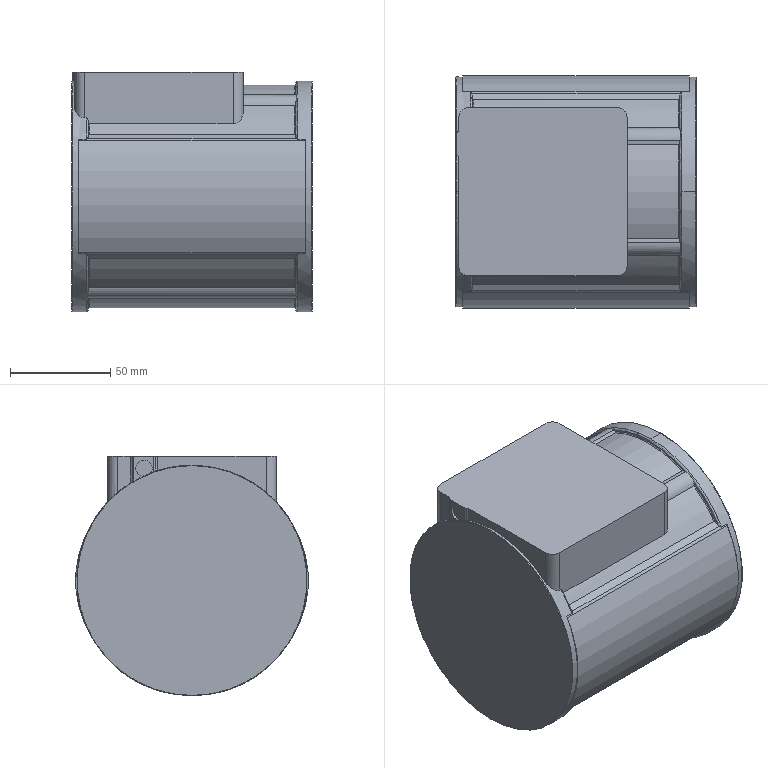Part | STEP file | G3L22N30-MM02TNNTNXH6-Part-6 | 1 solid | 96 faces | box 120 x 116.12 x 119.5 mm | volume 1293330 mm3 | cylinder 34 | plane 25 | torus 20 | cone 17 | commonest cylinder face diameters 111 x7 13 x6 115 x5 2 x4 6 x4 10 x4